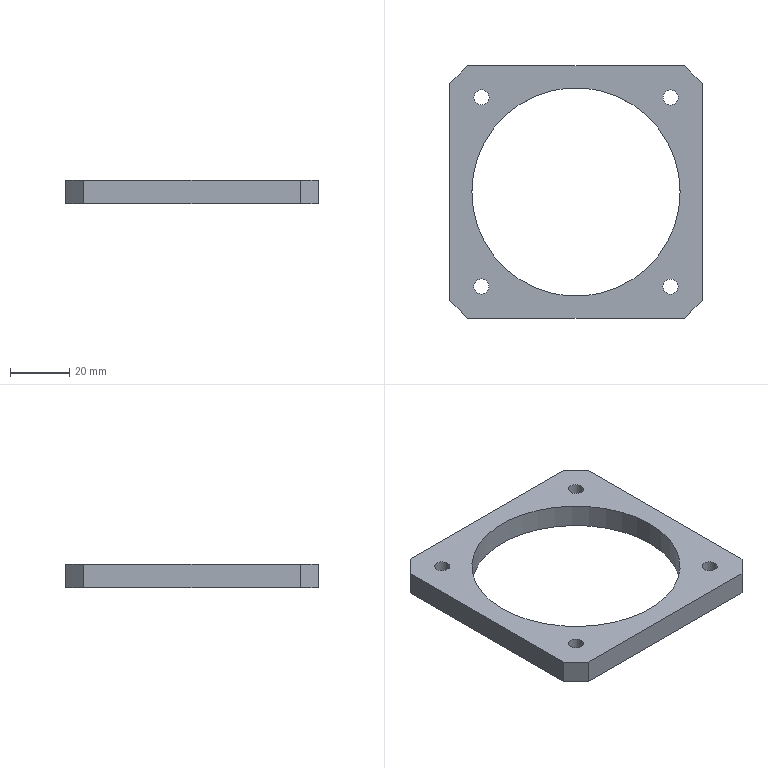CAM job | NX | 3-axis milling, drilling | part box 85 x 85 x 8 mm | stock box 92 x 92 x 8 mm
Tools:
number,name,description,diameter,corner_radius,flute_length,length,flutes
6,D4反刮刀,Milling Tool-5 Parameters,2.0,0.0,0.85,0.85,2
5,M6丝锥,Drilling Tool,6.0,0.0,35.0,50.0,2
4,D5钻头,Drilling Tool,5.1,0.0,35.0,50.0,2
3,D8.3,Drilling Tool,8.3,0.0,35.0,50.0,2
8,D63面刀,Milling Tool-5 Parameters,63.0,0.0,30.0,100.0,2
11,D50面刀,Milling Tool-5 Parameters,50.0,0.0,30.0,100.0,2
2,D10C-25L-35L,Milling Tool-5 Parameters,10.0,0.0,25.0,75.0,2
3,8J-20L-30L,Milling Tool-5 Parameters,8.0,0.0,20.0,65.0,2
7,D8点钻,Drilling Tool,8.0,0.0,10.0,75.0,2
Operations:
program,operation,operation_type,tool,method,geometry_group,spindle_rpm,surface_speed,feed_per_tooth,feed_cut,feed_plunge,cut_length_mm,path_length_mm,cut_time_min,machine_time_min
A0101,FACE_MILLING_COPY,FaceMilling,D63面刀,METHOD,W1,3500.0,692.0,0.1429,1000.0,100.0,434.0,718.49,0.434,0.4624
A0102,DRILLING,Operation,D8点钻,METHOD,W2,1200.0,30.0,0.1042,250.0,0.0,5.0,13.0,0.02,0.0208
G54,DRILLING_1,Operation,D8.3,METHOD,W2,1200.0,31.0,0.1042,250.0,0.0,15.0,33.0,0.06,0.0618
A0104,FACE_MILLING,FaceMilling,D63面刀,METHOD,W1,3500.0,692.0,0.1143,800.0,100.0,434.0,718.691,0.5425,0.571
B0101,ADAPTIVE_MILLING,CavityMilling,D10C-25L-35L,METHOD,W1,6500.0,204.0,0.1538,2000.0,100.0,1974.517,2026.517,0.9873,0.9925
B0101,PLANAR_MILL,PlanarMilling,8J-20L-30L,METHOD,W1,3500.0,109.0,0.1143,800.0,100.0,360.216,411.216,0.4503,0.4554
B0101,DRILLING_2,Operation,D8点钻,METHOD,W1,1200.0,30.0,0.0833,200.0,0.0,24.0,288.131,0.12,0.1464
B0101,DRILLING_2_COPY,Operation,D5钻头,METHOD,W1,1200.0,30.0,0.0833,200.0,0.0,64.0,368.131,0.32,0.3504
B0101,DRILLING_2_COPY_COPY,Operation,M6丝锥,METHOD,W1,400.0,7.0,0.5,400.0,0.0,60.0,360.131,0.15,0.18
B0101,PLANAR_MILL_1,PlanarMilling,D50面刀,METHOD,W1,3500.0,549.0,0.1143,800.0,100.0,386.447,420.347,0.4831,0.4864
B0101,PLANAR_MILL_1_COPY,PlanarMilling,D63面刀,METHOD,W1,3500.0,549.0,0.1143,800.0,100.0,427.288,461.288,0.5341,0.5375
B0101,PLANAR_MILL_2,PlanarMilling,D4反刮刀,METHOD,W1,3500.0,21.0,0.1429,1000.0,100.0,347.649,382.649,0.3476,0.3511
B0101,PLANAR_MILL_2_COPY,PlanarMilling,D4反刮刀,METHOD,W1,3500.0,21.0,0.1429,1000.0,100.0,349.848,401.548,0.3498,0.355
B0101,PLANAR_MILL_4,PlanarMilling,D4反刮刀,METHOD,W1,3500.0,21.0,0.1143,800.0,100.0,63.452,470.571,0.0793,0.12
B0102,PLANAR_MILL_3,PlanarMilling,D10C-25L-35L,METHOD,W1,4500.0,141.0,0.1667,1500.0,100.0,1565.983,1608.983,1.044,1.048
B0102,PLANAR_MILL_3_COPY_1,PlanarMilling,D10C-25L-35L,METHOD,W1,4500.0,141.0,0.1667,1500.0,100.0,3100.551,3232.576,2.067,2.08
B0102,PLANAR_MILL_3_COPY,PlanarMilling,8J-20L-30L,METHOD,W1,3500.0,109.0,0.1143,800.0,100.0,407.077,459.077,0.5088,0.514
B0102,PLANAR_MILL_2_COPY_1,PlanarMilling,D4反刮刀,METHOD,W1,3500.0,21.0,0.1429,1000.0,100.0,223.525,258.525,0.2235,0.227
B0102,PLANAR_MILL_2_COPY_COPY,PlanarMilling,D4反刮刀,METHOD,W1,3500.0,21.0,0.1429,1000.0,100.0,221.327,273.227,0.2213,0.2265